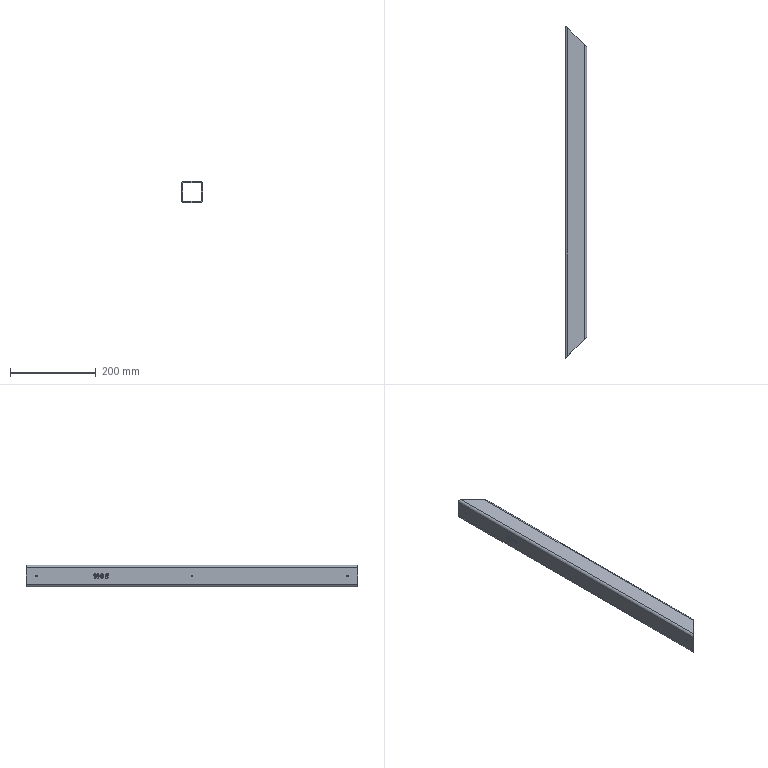Part | SolidWorks | features BaseBody 1 | 1 solid | 91 faces | box 50 x 773 x 50 mm | volume 392198 mm3 | plane 48 | spline 29 | cylinder 14 | commonest cylinder face diameters 4.2 x6 6 x4 12 x4